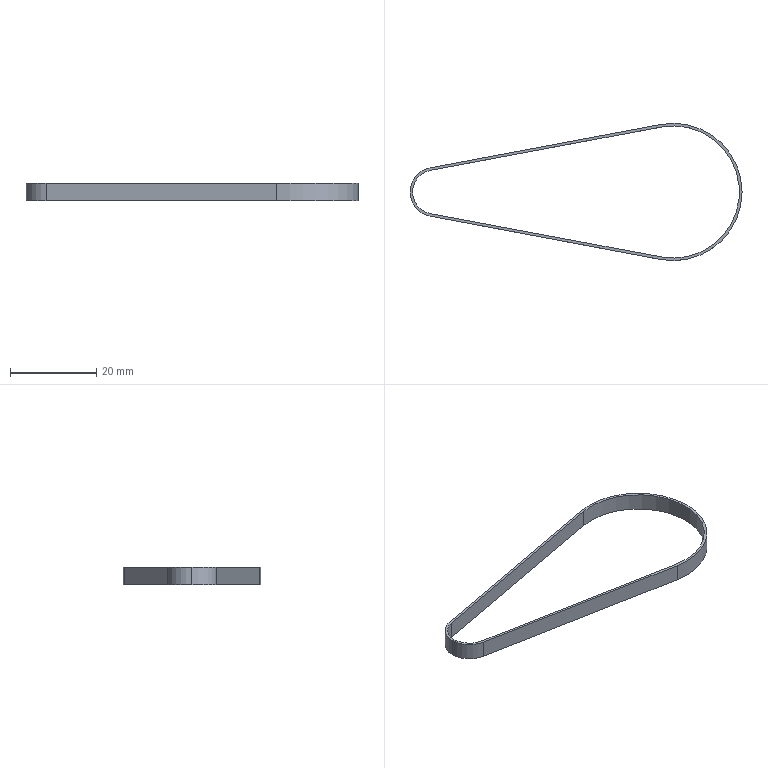Part | SolidWorks | features Extrusion 1 | 1 solid | 12 faces | box 76.775 x 31.76 x 4 mm | volume 427.631 mm3 | cylinder 6 | plane 6 | commonest cylinder face diameters 10.19 x2 11.39 x2 30.56 x1 31.76 x1
STEP:
#1=CARTESIAN_POINT('',(-0.9401,5.008,4.));
#2=VERTEX_POINT('',#1);
#3=CARTESIAN_POINT('',(-5.095,0.,4.));
#4=VERTEX_POINT('',#3);
#5=CARTESIAN_POINT('',(0.,0.,4.));
#6=DIRECTION('',(0.,0.,1.));
#7=DIRECTION('',(1.,0.,0.));
#8=AXIS2_PLACEMENT_3D('',#5,#6,#7);
#9=CIRCLE('',#8,5.095);
#10=EDGE_CURVE('',#2,#4,#9,.T.);
#11=ORIENTED_EDGE('',*,*,#10,.T.);
#12=CARTESIAN_POINT('',(-5.095,0.,0.));
#13=VERTEX_POINT('',#12);
#14=CARTESIAN_POINT('',(-5.095,0.,4.));
#15=DIRECTION('',(0.,0.,-1.));
#16=VECTOR('',#15,1000.);
#17=LINE('',#14,#16);
#18=EDGE_CURVE('',#4,#13,#17,.T.);
#19=ORIENTED_EDGE('',*,*,#18,.T.);
#20=CARTESIAN_POINT('',(-0.9401,5.008,0.));
#21=VERTEX_POINT('',#20);
#22=CARTESIAN_POINT('',(0.,0.,0.));
#23=DIRECTION('',(0.,0.,1.));
#24=DIRECTION('',(1.,0.,0.));
#25=AXIS2_PLACEMENT_3D('',#22,#23,#24);
#26=CIRCLE('',#25,5.095);
#27=EDGE_CURVE('',#21,#13,#26,.T.);
#28=ORIENTED_EDGE('',*,*,#27,.F.);
#29=CARTESIAN_POINT('',(-0.9401,5.008,4.));
#30=DIRECTION('',(0.,0.,-1.));
#31=VECTOR('',#30,1000.);
#32=LINE('',#29,#31);
#33=EDGE_CURVE('',#2,#21,#32,.T.);
#34=ORIENTED_EDGE('',*,*,#33,.F.);
#35=EDGE_LOOP('',(#11,#19,#28,#34));
#36=FACE_OUTER_BOUND('',#35,.T.);
#37=CARTESIAN_POINT('',(0.,0.,4.));
#38=DIRECTION('',(0.,0.,-1.));
#39=DIRECTION('',(-1.,0.,0.));
#40=AXIS2_PLACEMENT_3D('',#37,#38,#39);
#41=CYLINDRICAL_SURFACE('',#40,5.095);
#42=ADVANCED_FACE('',(#36),#41,.F.);
#43=CARTESIAN_POINT('',(-5.695,0.,4.));
#44=VERTEX_POINT('',#43);
#45=CARTESIAN_POINT('',(-1.051,-5.597,4.));
#46=VERTEX_POINT('',#45);
#47=CARTESIAN_POINT('',(0.,0.,4.));
#48=DIRECTION('',(0.,0.,1.));
#49=DIRECTION('',(1.,0.,0.));
#50=AXIS2_PLACEMENT_3D('',#47,#48,#49);
#51=CIRCLE('',#50,5.695);
#52=EDGE_CURVE('',#44,#46,#51,.T.);
#53=ORIENTED_EDGE('',*,*,#52,.F.);
#54=CARTESIAN_POINT('',(-5.695,0.,0.));
#55=VERTEX_POINT('',#54);
#56=CARTESIAN_POINT('',(-5.695,0.,4.));
#57=DIRECTION('',(0.,0.,-1.));
#58=VECTOR('',#57,1000.);
#59=LINE('',#56,#58);
#60=EDGE_CURVE('',#44,#55,#59,.T.);
#61=ORIENTED_EDGE('',*,*,#60,.T.);
#62=CARTESIAN_POINT('',(-1.051,-5.597,0.));
#63=VERTEX_POINT('',#62);
#64=CARTESIAN_POINT('',(0.,0.,0.));
#65=DIRECTION('',(0.,0.,1.));
#66=DIRECTION('',(1.,0.,0.));
#67=AXIS2_PLACEMENT_3D('',#64,#65,#66);
#68=CIRCLE('',#67,5.695);
#69=EDGE_CURVE('',#55,#63,#68,.T.);
#70=ORIENTED_EDGE('',*,*,#69,.T.);
#71=CARTESIAN_POINT('',(-1.051,-5.597,4.));
#72=DIRECTION('',(0.,0.,-1.));
#73=VECTOR('',#72,1000.);
#74=LINE('',#71,#73);
#75=EDGE_CURVE('',#46,#63,#74,.T.);
#76=ORIENTED_EDGE('',*,*,#75,.F.);
#77=EDGE_LOOP('',(#53,#61,#70,#76));
#78=FACE_OUTER_BOUND('',#77,.T.);
#79=CARTESIAN_POINT('',(0.,0.,4.));
#80=DIRECTION('',(0.,0.,-1.));
#81=DIRECTION('',(-1.,0.,0.));
#82=AXIS2_PLACEMENT_3D('',#79,#80,#81);
#83=CYLINDRICAL_SURFACE('',#82,5.695);
#84=ADVANCED_FACE('',(#78),#83,.T.);
#85=CARTESIAN_POINT('',(-1.051,5.597,4.));
#86=VERTEX_POINT('',#85);
#87=CARTESIAN_POINT('',(0.,0.,4.));
#88=DIRECTION('',(0.,0.,1.));
#89=DIRECTION('',(1.,0.,0.));
#90=AXIS2_PLACEMENT_3D('',#87,#88,#89);
#91=CIRCLE('',#90,5.695);
#92=EDGE_CURVE('',#86,#44,#91,.T.);
#93=ORIENTED_EDGE('',*,*,#92,.T.);
#94=ORIENTED_EDGE('',*,*,#52,.T.);
#95=CARTESIAN_POINT('',(52.27,-15.607,4.));
#96=VERTEX_POINT('',#95);
#97=CARTESIAN_POINT('',(-1.051,-5.597,4.));
#98=DIRECTION('',(0.9828,-0.1845,0.));
#99=VECTOR('',#98,1000.);
#100=LINE('',#97,#99);
#101=EDGE_CURVE('',#46,#96,#100,.T.);
#102=ORIENTED_EDGE('',*,*,#101,.T.);
#103=CARTESIAN_POINT('',(52.27,15.607,4.));
#104=VERTEX_POINT('',#103);
#105=CARTESIAN_POINT('',(55.2,0.,4.));
#106=DIRECTION('',(0.,0.,1.));
#107=DIRECTION('',(1.,0.,0.));
#108=AXIS2_PLACEMENT_3D('',#105,#106,#107);
#109=CIRCLE('',#108,15.88);
#110=EDGE_CURVE('',#96,#104,#109,.T.);
#111=ORIENTED_EDGE('',*,*,#110,.T.);
#112=CARTESIAN_POINT('',(-1.051,5.597,4.));
#113=DIRECTION('',(-0.9828,-0.1845,0.));
#114=VECTOR('',#113,1000.);
#115=LINE('',#112,#114);
#116=EDGE_CURVE('',#104,#86,#115,.T.);
#117=ORIENTED_EDGE('',*,*,#116,.T.);
#118=EDGE_LOOP('',(#93,#94,#102,#111,#117));
#119=FACE_OUTER_BOUND('',#118,.T.);
#120=CARTESIAN_POINT('',(-0.9401,-5.008,4.));
#121=VERTEX_POINT('',#120);
#122=CARTESIAN_POINT('',(52.381,-15.018,4.));
#123=VERTEX_POINT('',#122);
#124=CARTESIAN_POINT('',(-0.9401,-5.008,4.));
#125=DIRECTION('',(0.9828,-0.1845,0.));
#126=VECTOR('',#125,1000.);
#127=LINE('',#124,#126);
#128=EDGE_CURVE('',#121,#123,#127,.T.);
#129=ORIENTED_EDGE('',*,*,#128,.F.);
#130=CARTESIAN_POINT('',(0.,0.,4.));
#131=DIRECTION('',(0.,0.,1.));
#132=DIRECTION('',(1.,0.,0.));
#133=AXIS2_PLACEMENT_3D('',#130,#131,#132);
#134=CIRCLE('',#133,5.095);
#135=EDGE_CURVE('',#4,#121,#134,.T.);
#136=ORIENTED_EDGE('',*,*,#135,.F.);
#137=ORIENTED_EDGE('',*,*,#10,.F.);
#138=CARTESIAN_POINT('',(52.381,15.018,4.));
#139=VERTEX_POINT('',#138);
#140=CARTESIAN_POINT('',(-0.9401,5.008,4.));
#141=DIRECTION('',(-0.9828,-0.1845,0.));
#142=VECTOR('',#141,1000.);
#143=LINE('',#140,#142);
#144=EDGE_CURVE('',#139,#2,#143,.T.);
#145=ORIENTED_EDGE('',*,*,#144,.F.);
#146=CARTESIAN_POINT('',(55.2,0.,4.));
#147=DIRECTION('',(0.,0.,1.));
#148=DIRECTION('',(1.,0.,0.));
#149=AXIS2_PLACEMENT_3D('',#146,#147,#148);
#150=CIRCLE('',#149,15.28);
#151=EDGE_CURVE('',#123,#139,#150,.T.);
#152=ORIENTED_EDGE('',*,*,#151,.F.);
#153=EDGE_LOOP('',(#129,#136,#137,#145,#152));
#154=FACE_BOUND('',#153,.T.);
#155=CARTESIAN_POINT('',(0.,0.,4.));
#156=DIRECTION('',(0.,0.,1.));
#157=DIRECTION('',(1.,0.,0.));
#158=AXIS2_PLACEMENT_3D('',#155,#156,#157);
#159=PLANE('',#158);
#160=ADVANCED_FACE('',(#119,#154),#159,.T.);
#161=CARTESIAN_POINT('',(-1.051,5.597,0.));
#162=VERTEX_POINT('',#161);
#163=CARTESIAN_POINT('',(0.,0.,0.));
#164=DIRECTION('',(0.,0.,1.));
#165=DIRECTION('',(1.,0.,0.));
#166=AXIS2_PLACEMENT_3D('',#163,#164,#165);
#167=CIRCLE('',#166,5.695);
#168=EDGE_CURVE('',#162,#55,#167,.T.);
#169=ORIENTED_EDGE('',*,*,#168,.F.);
#170=CARTESIAN_POINT('',(52.27,15.607,0.));
#171=VERTEX_POINT('',#170);
#172=CARTESIAN_POINT('',(-1.051,5.597,0.));
#173=DIRECTION('',(-0.9828,-0.1845,0.));
#174=VECTOR('',#173,1000.);
#175=LINE('',#172,#174);
#176=EDGE_CURVE('',#171,#162,#175,.T.);
#177=ORIENTED_EDGE('',*,*,#176,.F.);
#178=CARTESIAN_POINT('',(52.27,-15.607,0.));
#179=VERTEX_POINT('',#178);
#180=CARTESIAN_POINT('',(55.2,0.,0.));
#181=DIRECTION('',(0.,0.,1.));
#182=DIRECTION('',(1.,0.,0.));
#183=AXIS2_PLACEMENT_3D('',#180,#181,#182);
#184=CIRCLE('',#183,15.88);
#185=EDGE_CURVE('',#179,#171,#184,.T.);
#186=ORIENTED_EDGE('',*,*,#185,.F.);
#187=CARTESIAN_POINT('',(-1.051,-5.597,0.));
#188=DIRECTION('',(0.9828,-0.1845,0.));
#189=VECTOR('',#188,1000.);
#190=LINE('',#187,#189);
#191=EDGE_CURVE('',#63,#179,#190,.T.);
#192=ORIENTED_EDGE('',*,*,#191,.F.);
#193=ORIENTED_EDGE('',*,*,#69,.F.);
#194=EDGE_LOOP('',(#169,#177,#186,#192,#193));
#195=FACE_OUTER_BOUND('',#194,.T.);
#196=ORIENTED_EDGE('',*,*,#27,.T.);
#197=CARTESIAN_POINT('',(-0.9401,-5.008,0.));
#198=VERTEX_POINT('',#197);
#199=CARTESIAN_POINT('',(0.,0.,0.));
#200=DIRECTION('',(0.,0.,1.));
#201=DIRECTION('',(1.,0.,0.));
#202=AXIS2_PLACEMENT_3D('',#199,#200,#201);
#203=CIRCLE('',#202,5.095);
#204=EDGE_CURVE('',#13,#198,#203,.T.);
#205=ORIENTED_EDGE('',*,*,#204,.T.);
#206=CARTESIAN_POINT('',(52.381,-15.018,0.));
#207=VERTEX_POINT('',#206);
#208=CARTESIAN_POINT('',(-0.9401,-5.008,0.));
#209=DIRECTION('',(0.9828,-0.1845,0.));
#210=VECTOR('',#209,1000.);
#211=LINE('',#208,#210);
#212=EDGE_CURVE('',#198,#207,#211,.T.);
#213=ORIENTED_EDGE('',*,*,#212,.T.);
#214=CARTESIAN_POINT('',(52.381,15.018,0.));
#215=VERTEX_POINT('',#214);
#216=CARTESIAN_POINT('',(55.2,0.,0.));
#217=DIRECTION('',(0.,0.,1.));
#218=DIRECTION('',(1.,0.,0.));
#219=AXIS2_PLACEMENT_3D('',#216,#217,#218);
#220=CIRCLE('',#219,15.28);
#221=EDGE_CURVE('',#207,#215,#220,.T.);
#222=ORIENTED_EDGE('',*,*,#221,.T.);
#223=CARTESIAN_POINT('',(-0.9401,5.008,0.));
#224=DIRECTION('',(-0.9828,-0.1845,0.));
#225=VECTOR('',#224,1000.);
#226=LINE('',#223,#225);
#227=EDGE_CURVE('',#215,#21,#226,.T.);
#228=ORIENTED_EDGE('',*,*,#227,.T.);
#229=EDGE_LOOP('',(#196,#205,#213,#222,#228));
#230=FACE_BOUND('',#229,.T.);
#231=CARTESIAN_POINT('',(0.,0.,0.));
#232=DIRECTION('',(0.,0.,1.));
#233=DIRECTION('',(1.,0.,0.));
#234=AXIS2_PLACEMENT_3D('',#231,#232,#233);
#235=PLANE('',#234);
#236=ADVANCED_FACE('',(#195,#230),#235,.F.);
#237=ORIENTED_EDGE('',*,*,#60,.F.);
#238=ORIENTED_EDGE('',*,*,#92,.F.);
#239=CARTESIAN_POINT('',(-1.051,5.597,4.));
#240=DIRECTION('',(0.,0.,-1.));
#241=VECTOR('',#240,1000.);
#242=LINE('',#239,#241);
#243=EDGE_CURVE('',#86,#162,#242,.T.);
#244=ORIENTED_EDGE('',*,*,#243,.T.);
#245=ORIENTED_EDGE('',*,*,#168,.T.);
#246=EDGE_LOOP('',(#237,#238,#244,#245));
#247=FACE_OUTER_BOUND('',#246,.T.);
#248=CARTESIAN_POINT('',(0.,0.,4.));
#249=DIRECTION('',(0.,0.,-1.));
#250=DIRECTION('',(-1.,0.,0.));
#251=AXIS2_PLACEMENT_3D('',#248,#249,#250);
#252=CYLINDRICAL_SURFACE('',#251,5.695);
#253=ADVANCED_FACE('',(#247),#252,.T.);
#254=ORIENTED_EDGE('',*,*,#191,.T.);
#255=CARTESIAN_POINT('',(52.27,-15.607,4.));
#256=DIRECTION('',(0.,0.,-1.));
#257=VECTOR('',#256,1000.);
#258=LINE('',#255,#257);
#259=EDGE_CURVE('',#96,#179,#258,.T.);
#260=ORIENTED_EDGE('',*,*,#259,.F.);
#261=ORIENTED_EDGE('',*,*,#101,.F.);
#262=ORIENTED_EDGE('',*,*,#75,.T.);
#263=EDGE_LOOP('',(#254,#260,#261,#262));
#264=FACE_OUTER_BOUND('',#263,.T.);
#265=CARTESIAN_POINT('',(-1.051,-5.597,4.));
#266=DIRECTION('',(0.1845,0.9828,0.));
#267=DIRECTION('',(-0.9828,0.1845,0.));
#268=AXIS2_PLACEMENT_3D('',#265,#266,#267);
#269=PLANE('',#268);
#270=ADVANCED_FACE('',(#264),#269,.F.);
#271=ORIENTED_EDGE('',*,*,#185,.T.);
#272=CARTESIAN_POINT('',(52.27,15.607,4.));
#273=DIRECTION('',(0.,0.,-1.));
#274=VECTOR('',#273,1000.);
#275=LINE('',#272,#274);
#276=EDGE_CURVE('',#104,#171,#275,.T.);
#277=ORIENTED_EDGE('',*,*,#276,.F.);
#278=ORIENTED_EDGE('',*,*,#110,.F.);
#279=ORIENTED_EDGE('',*,*,#259,.T.);
#280=EDGE_LOOP('',(#271,#277,#278,#279));
#281=FACE_OUTER_BOUND('',#280,.T.);
#282=CARTESIAN_POINT('',(55.2,0.,4.));
#283=DIRECTION('',(0.,0.,-1.));
#284=DIRECTION('',(-1.,0.,0.));
#285=AXIS2_PLACEMENT_3D('',#282,#283,#284);
#286=CYLINDRICAL_SURFACE('',#285,15.88);
#287=ADVANCED_FACE('',(#281),#286,.T.);
#288=ORIENTED_EDGE('',*,*,#176,.T.);
#289=ORIENTED_EDGE('',*,*,#243,.F.);
#290=ORIENTED_EDGE('',*,*,#116,.F.);
#291=ORIENTED_EDGE('',*,*,#276,.T.);
#292=EDGE_LOOP('',(#288,#289,#290,#291));
#293=FACE_OUTER_BOUND('',#292,.T.);
#294=CARTESIAN_POINT('',(-1.051,5.597,4.));
#295=DIRECTION('',(0.1845,-0.9828,0.));
#296=DIRECTION('',(0.9828,0.1845,0.));
#297=AXIS2_PLACEMENT_3D('',#294,#295,#296);
#298=PLANE('',#297);
#299=ADVANCED_FACE('',(#293),#298,.F.);
#300=ORIENTED_EDGE('',*,*,#18,.F.);
#301=ORIENTED_EDGE('',*,*,#135,.T.);
#302=CARTESIAN_POINT('',(-0.9401,-5.008,4.));
#303=DIRECTION('',(0.,0.,-1.));
#304=VECTOR('',#303,1000.);
#305=LINE('',#302,#304);
#306=EDGE_CURVE('',#121,#198,#305,.T.);
#307=ORIENTED_EDGE('',*,*,#306,.T.);
#308=ORIENTED_EDGE('',*,*,#204,.F.);
#309=EDGE_LOOP('',(#300,#301,#307,#308));
#310=FACE_OUTER_BOUND('',#309,.T.);
#311=CARTESIAN_POINT('',(0.,0.,4.));
#312=DIRECTION('',(0.,0.,-1.));
#313=DIRECTION('',(-1.,0.,0.));
#314=AXIS2_PLACEMENT_3D('',#311,#312,#313);
#315=CYLINDRICAL_SURFACE('',#314,5.095);
#316=ADVANCED_FACE('',(#310),#315,.F.);
#317=ORIENTED_EDGE('',*,*,#212,.F.);
#318=ORIENTED_EDGE('',*,*,#306,.F.);
#319=ORIENTED_EDGE('',*,*,#128,.T.);
#320=CARTESIAN_POINT('',(52.381,-15.018,4.));
#321=DIRECTION('',(0.,0.,-1.));
#322=VECTOR('',#321,1000.);
#323=LINE('',#320,#322);
#324=EDGE_CURVE('',#123,#207,#323,.T.);
#325=ORIENTED_EDGE('',*,*,#324,.T.);
#326=EDGE_LOOP('',(#317,#318,#319,#325));
#327=FACE_OUTER_BOUND('',#326,.T.);
#328=CARTESIAN_POINT('',(-0.9401,-5.008,4.));
#329=DIRECTION('',(0.1845,0.9828,0.));
#330=DIRECTION('',(-0.9828,0.1845,0.));
#331=AXIS2_PLACEMENT_3D('',#328,#329,#330);
#332=PLANE('',#331);
#333=ADVANCED_FACE('',(#327),#332,.T.);
#334=ORIENTED_EDGE('',*,*,#221,.F.);
#335=ORIENTED_EDGE('',*,*,#324,.F.);
#336=ORIENTED_EDGE('',*,*,#151,.T.);
#337=CARTESIAN_POINT('',(52.381,15.018,4.));
#338=DIRECTION('',(0.,0.,-1.));
#339=VECTOR('',#338,1000.);
#340=LINE('',#337,#339);
#341=EDGE_CURVE('',#139,#215,#340,.T.);
#342=ORIENTED_EDGE('',*,*,#341,.T.);
#343=EDGE_LOOP('',(#334,#335,#336,#342));
#344=FACE_OUTER_BOUND('',#343,.T.);
#345=CARTESIAN_POINT('',(55.2,0.,4.));
#346=DIRECTION('',(0.,0.,-1.));
#347=DIRECTION('',(-1.,0.,0.));
#348=AXIS2_PLACEMENT_3D('',#345,#346,#347);
#349=CYLINDRICAL_SURFACE('',#348,15.28);
#350=ADVANCED_FACE('',(#344),#349,.F.);
#351=ORIENTED_EDGE('',*,*,#227,.F.);
#352=ORIENTED_EDGE('',*,*,#341,.F.);
#353=ORIENTED_EDGE('',*,*,#144,.T.);
#354=ORIENTED_EDGE('',*,*,#33,.T.);
#355=EDGE_LOOP('',(#351,#352,#353,#354));
#356=FACE_OUTER_BOUND('',#355,.T.);
#357=CARTESIAN_POINT('',(-0.9401,5.008,4.));
#358=DIRECTION('',(0.1845,-0.9828,0.));
#359=DIRECTION('',(0.9828,0.1845,0.));
#360=AXIS2_PLACEMENT_3D('',#357,#358,#359);
#361=PLANE('',#360);
#362=ADVANCED_FACE('',(#356),#361,.T.);
#363=CLOSED_SHELL('',(#42,#84,#160,#236,#253,#270,#287,#299,#316,#333,#350,#362));
#364=MANIFOLD_SOLID_BREP('',#363);
#365=CARTESIAN_POINT('',(0.,0.,0.));
#366=DIRECTION('',(0.,0.,1.));
#367=DIRECTION('',(1.,0.,0.));
#368=AXIS2_PLACEMENT_3D('',#365,#366,#367);
#369=(LENGTH_UNIT()NAMED_UNIT(*)SI_UNIT(.MILLI.,.METRE.));
#370=UNCERTAINTY_MEASURE_WITH_UNIT(LENGTH_MEASURE(0.00001),#369,'','');
#371=(NAMED_UNIT(*)PLANE_ANGLE_UNIT()SI_UNIT($,.RADIAN.));
#372=(NAMED_UNIT(*)SI_UNIT($,.STERADIAN.)SOLID_ANGLE_UNIT());
#373=(GEOMETRIC_REPRESENTATION_CONTEXT(3)GLOBAL_UNCERTAINTY_ASSIGNED_CONTEXT((#370))GLOBAL_UNIT_ASSIGNED_CONTEXT((#369,#371,#372))REPRESENTATION_CONTEXT('',''));
#374=ADVANCED_BREP_SHAPE_REPRESENTATION('',(#364,#368),#373);